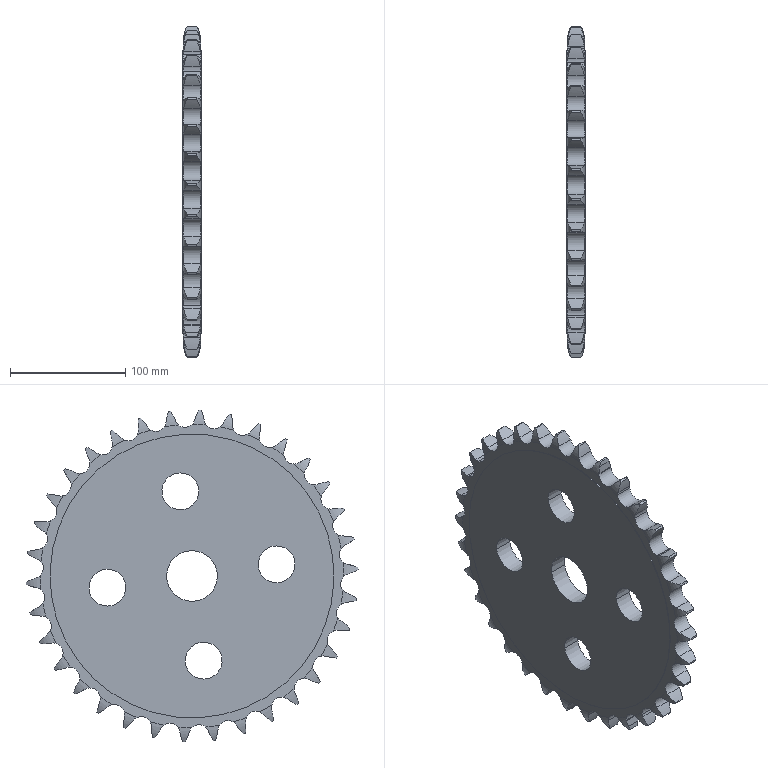Part | STEP file | Cut-Extrude 4-1 | 1 solid | 242 faces | box 16 x 287.619 x 287.573 mm | volume 813430 mm3 | cylinder 170 | torus 68 | plane 4 | commonest cylinder face diameters 137.203 x72 17.468 x50 287.826 x34 32 x8 246 x4 44 x2